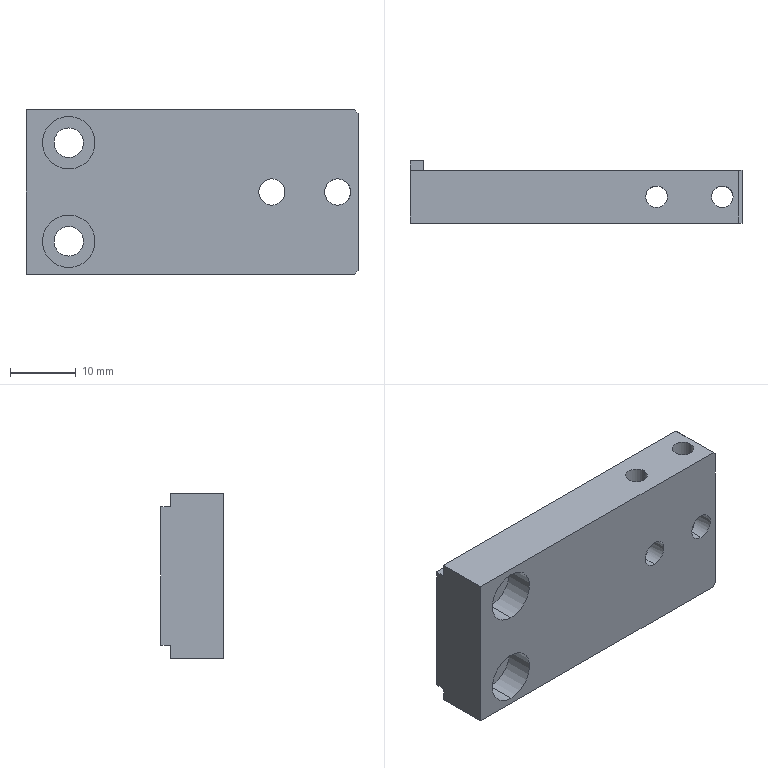Part | STEP file | 11-FG-B07811 | 1 solid | 34 faces | box 50.5 x 9.5 x 25 mm | volume 9037 mm3 | cylinder 20 | plane 14 | commonest cylinder face diameters 3.3 x8 4 x4 4.5 x4 8 x4
STEP:
#1=CARTESIAN_POINT('',(33.85,0.,1.264));
#2=VERTEX_POINT('',#1);
#3=CARTESIAN_POINT('',(35.4,-1.647,2.));
#4=VERTEX_POINT('',#3);
#5=CARTESIAN_POINT('',(33.85,0.,1.264));
#6=CARTESIAN_POINT('',(33.85,-0.2198,1.264));
#7=CARTESIAN_POINT('',(33.895,-0.4332,1.322));
#8=CARTESIAN_POINT('',(34.01,-0.7157,1.439));
#9=CARTESIAN_POINT('',(34.057,-0.8056,1.483));
#10=CARTESIAN_POINT('',(34.163,-0.9726,1.573));
#11=CARTESIAN_POINT('',(34.224,-1.05,1.619));
#12=CARTESIAN_POINT('',(34.358,-1.195,1.709));
#13=CARTESIAN_POINT('',(34.434,-1.263,1.753));
#14=CARTESIAN_POINT('',(34.596,-1.384,1.834));
#15=CARTESIAN_POINT('',(34.684,-1.438,1.87));
#16=CARTESIAN_POINT('',(34.967,-1.575,1.963));
#17=CARTESIAN_POINT('',(35.18,-1.634,2.));
#18=CARTESIAN_POINT('',(35.4,-1.647,2.));
#19=B_SPLINE_CURVE_WITH_KNOTS('',3,(#5,#6,#7,#8,#9,#10,#11,#12,#13,#14,#15,#16,#17,#18),.UNSPECIFIED.,.F.,.F.,(4,2,2,2,2,2,4),(0.008422,0.009072,0.009397,0.009722,0.01005,0.01037,0.01102),.UNSPECIFIED.);
#20=EDGE_CURVE('',#2,#4,#19,.T.);
#21=ORIENTED_EDGE('',*,*,#20,.F.);
#22=CARTESIAN_POINT('',(33.85,0.,12.5));
#23=VERTEX_POINT('',#22);
#24=CARTESIAN_POINT('',(33.85,0.,12.5));
#25=DIRECTION('',(0.,0.,1.));
#26=VECTOR('',#25,1000.);
#27=LINE('',#24,#26);
#28=EDGE_CURVE('',#2,#23,#27,.T.);
#29=ORIENTED_EDGE('',*,*,#28,.T.);
#30=CARTESIAN_POINT('',(37.15,0.,12.5));
#31=VERTEX_POINT('',#30);
#32=CARTESIAN_POINT('',(35.5,0.,12.5));
#33=DIRECTION('',(0.,0.,1.));
#34=DIRECTION('',(1.,0.,0.));
#35=AXIS2_PLACEMENT_3D('',#32,#33,#34);
#36=CIRCLE('',#35,1.65);
#37=EDGE_CURVE('',#23,#31,#36,.T.);
#38=ORIENTED_EDGE('',*,*,#37,.T.);
#39=CARTESIAN_POINT('',(37.15,0.,0.9682));
#40=VERTEX_POINT('',#39);
#41=CARTESIAN_POINT('',(37.15,0.,12.5));
#42=DIRECTION('',(0.,0.,1.));
#43=VECTOR('',#42,1000.);
#44=LINE('',#41,#43);
#45=EDGE_CURVE('',#40,#31,#44,.T.);
#46=ORIENTED_EDGE('',*,*,#45,.F.);
#47=CARTESIAN_POINT('',(35.4,-1.647,2.));
#48=CARTESIAN_POINT('',(35.523,-1.654,2.));
#49=CARTESIAN_POINT('',(35.643,-1.648,1.989));
#50=CARTESIAN_POINT('',(35.88,-1.61,1.945));
#51=CARTESIAN_POINT('',(35.995,-1.578,1.913));
#52=CARTESIAN_POINT('',(36.208,-1.495,1.833));
#53=CARTESIAN_POINT('',(36.309,-1.442,1.784));
#54=CARTESIAN_POINT('',(36.492,-1.323,1.679));
#55=CARTESIAN_POINT('',(36.575,-1.256,1.621));
#56=CARTESIAN_POINT('',(36.726,-1.109,1.5));
#57=CARTESIAN_POINT('',(36.794,-1.029,1.436));
#58=CARTESIAN_POINT('',(36.913,-0.8585,1.311));
#59=CARTESIAN_POINT('',(36.964,-0.7681,1.248));
#60=CARTESIAN_POINT('',(37.051,-0.572,1.131));
#61=CARTESIAN_POINT('',(37.086,-0.4683,1.076));
#62=CARTESIAN_POINT('',(37.136,-0.2428,0.9941));
#63=CARTESIAN_POINT('',(37.15,-0.1222,0.9682));
#64=CARTESIAN_POINT('',(37.15,0.,0.9682));
#65=B_SPLINE_CURVE_WITH_KNOTS('',3,(#47,#48,#49,#50,#51,#52,#53,#54,#55,#56,#57,#58,#59,#60,#61,#62,#63,#64),.UNSPECIFIED.,.F.,.F.,(4,2,2,2,2,2,2,2,4),(0.,0.0003631,0.0007262,0.001089,0.001452,0.001815,0.002179,0.002542,0.002905),.UNSPECIFIED.);
#66=EDGE_CURVE('',#4,#40,#65,.T.);
#67=ORIENTED_EDGE('',*,*,#66,.F.);
#68=EDGE_LOOP('',(#21,#29,#38,#46,#67));
#69=FACE_OUTER_BOUND('',#68,.T.);
#70=CARTESIAN_POINT('',(35.5,0.,12.5));
#71=DIRECTION('',(0.,0.,1.));
#72=DIRECTION('',(1.,0.,0.));
#73=AXIS2_PLACEMENT_3D('',#70,#71,#72);
#74=CYLINDRICAL_SURFACE('',#73,1.65);
#75=ADVANCED_FACE('',(#69),#74,.F.);
#76=CARTESIAN_POINT('',(43.85,0.,1.264));
#77=VERTEX_POINT('',#76);
#78=CARTESIAN_POINT('',(45.4,-1.647,2.));
#79=VERTEX_POINT('',#78);
#80=CARTESIAN_POINT('',(43.85,0.,1.264));
#81=CARTESIAN_POINT('',(43.85,-0.2198,1.264));
#82=CARTESIAN_POINT('',(43.895,-0.4332,1.322));
#83=CARTESIAN_POINT('',(44.01,-0.7157,1.439));
#84=CARTESIAN_POINT('',(44.057,-0.8056,1.483));
#85=CARTESIAN_POINT('',(44.163,-0.9726,1.573));
#86=CARTESIAN_POINT('',(44.224,-1.05,1.619));
#87=CARTESIAN_POINT('',(44.358,-1.195,1.709));
#88=CARTESIAN_POINT('',(44.434,-1.263,1.753));
#89=CARTESIAN_POINT('',(44.596,-1.384,1.834));
#90=CARTESIAN_POINT('',(44.684,-1.438,1.87));
#91=CARTESIAN_POINT('',(44.967,-1.575,1.963));
#92=CARTESIAN_POINT('',(45.18,-1.634,2.));
#93=CARTESIAN_POINT('',(45.4,-1.647,2.));
#94=B_SPLINE_CURVE_WITH_KNOTS('',3,(#80,#81,#82,#83,#84,#85,#86,#87,#88,#89,#90,#91,#92,#93),.UNSPECIFIED.,.F.,.F.,(4,2,2,2,2,2,4),(0.008422,0.009072,0.009397,0.009722,0.01005,0.01037,0.01102),.UNSPECIFIED.);
#95=EDGE_CURVE('',#77,#79,#94,.T.);
#96=ORIENTED_EDGE('',*,*,#95,.F.);
#97=CARTESIAN_POINT('',(43.85,0.,12.5));
#98=VERTEX_POINT('',#97);
#99=CARTESIAN_POINT('',(43.85,0.,12.5));
#100=DIRECTION('',(0.,0.,1.));
#101=VECTOR('',#100,1000.);
#102=LINE('',#99,#101);
#103=EDGE_CURVE('',#77,#98,#102,.T.);
#104=ORIENTED_EDGE('',*,*,#103,.T.);
#105=CARTESIAN_POINT('',(47.15,0.,12.5));
#106=VERTEX_POINT('',#105);
#107=CARTESIAN_POINT('',(45.5,0.,12.5));
#108=DIRECTION('',(0.,0.,1.));
#109=DIRECTION('',(1.,0.,0.));
#110=AXIS2_PLACEMENT_3D('',#107,#108,#109);
#111=CIRCLE('',#110,1.65);
#112=EDGE_CURVE('',#98,#106,#111,.T.);
#113=ORIENTED_EDGE('',*,*,#112,.T.);
#114=CARTESIAN_POINT('',(47.15,0.,0.9682));
#115=VERTEX_POINT('',#114);
#116=CARTESIAN_POINT('',(47.15,0.,12.5));
#117=DIRECTION('',(0.,0.,1.));
#118=VECTOR('',#117,1000.);
#119=LINE('',#116,#118);
#120=EDGE_CURVE('',#115,#106,#119,.T.);
#121=ORIENTED_EDGE('',*,*,#120,.F.);
#122=CARTESIAN_POINT('',(45.4,-1.647,2.));
#123=CARTESIAN_POINT('',(45.523,-1.654,2.));
#124=CARTESIAN_POINT('',(45.643,-1.648,1.989));
#125=CARTESIAN_POINT('',(45.88,-1.61,1.945));
#126=CARTESIAN_POINT('',(45.995,-1.578,1.913));
#127=CARTESIAN_POINT('',(46.208,-1.495,1.833));
#128=CARTESIAN_POINT('',(46.309,-1.442,1.784));
#129=CARTESIAN_POINT('',(46.492,-1.323,1.679));
#130=CARTESIAN_POINT('',(46.575,-1.256,1.621));
#131=CARTESIAN_POINT('',(46.726,-1.109,1.5));
#132=CARTESIAN_POINT('',(46.794,-1.029,1.436));
#133=CARTESIAN_POINT('',(46.913,-0.8585,1.311));
#134=CARTESIAN_POINT('',(46.964,-0.7681,1.248));
#135=CARTESIAN_POINT('',(47.051,-0.572,1.131));
#136=CARTESIAN_POINT('',(47.086,-0.4683,1.076));
#137=CARTESIAN_POINT('',(47.136,-0.2428,0.9941));
#138=CARTESIAN_POINT('',(47.15,-0.1222,0.9682));
#139=CARTESIAN_POINT('',(47.15,0.,0.9682));
#140=B_SPLINE_CURVE_WITH_KNOTS('',3,(#122,#123,#124,#125,#126,#127,#128,#129,#130,#131,#132,#133,#134,#135,#136,#137,#138,#139),.UNSPECIFIED.,.F.,.F.,(4,2,2,2,2,2,2,2,4),(0.,0.0003631,0.0007262,0.001089,0.001452,0.001815,0.002179,0.002542,0.002905),.UNSPECIFIED.);
#141=EDGE_CURVE('',#79,#115,#140,.T.);
#142=ORIENTED_EDGE('',*,*,#141,.F.);
#143=EDGE_LOOP('',(#96,#104,#113,#121,#142));
#144=FACE_OUTER_BOUND('',#143,.T.);
#145=CARTESIAN_POINT('',(45.5,0.,12.5));
#146=DIRECTION('',(0.,0.,1.));
#147=DIRECTION('',(1.,0.,0.));
#148=AXIS2_PLACEMENT_3D('',#145,#146,#147);
#149=CYLINDRICAL_SURFACE('',#148,1.65);
#150=ADVANCED_FACE('',(#144),#149,.F.);
#151=CARTESIAN_POINT('',(37.15,0.,-0.9682));
#152=VERTEX_POINT('',#151);
#153=CARTESIAN_POINT('',(35.4,-1.647,-2.));
#154=VERTEX_POINT('',#153);
#155=CARTESIAN_POINT('',(37.15,0.,-0.9682));
#156=CARTESIAN_POINT('',(37.15,-0.1224,-0.9682));
#157=CARTESIAN_POINT('',(37.136,-0.2437,-0.9944));
#158=CARTESIAN_POINT('',(37.086,-0.4679,-1.076));
#159=CARTESIAN_POINT('',(37.051,-0.5725,-1.131));
#160=CARTESIAN_POINT('',(36.964,-0.7681,-1.248));
#161=CARTESIAN_POINT('',(36.913,-0.8583,-1.311));
#162=CARTESIAN_POINT('',(36.794,-1.029,-1.436));
#163=CARTESIAN_POINT('',(36.726,-1.109,-1.5));
#164=CARTESIAN_POINT('',(36.575,-1.256,-1.621));
#165=CARTESIAN_POINT('',(36.492,-1.323,-1.679));
#166=CARTESIAN_POINT('',(36.31,-1.441,-1.784));
#167=CARTESIAN_POINT('',(36.209,-1.494,-1.832));
#168=CARTESIAN_POINT('',(35.888,-1.62,-1.953));
#169=CARTESIAN_POINT('',(35.643,-1.662,-2.));
#170=CARTESIAN_POINT('',(35.4,-1.647,-2.));
#171=B_SPLINE_CURVE_WITH_KNOTS('',3,(#155,#156,#157,#158,#159,#160,#161,#162,#163,#164,#165,#166,#167,#168,#169,#170),.UNSPECIFIED.,.F.,.F.,(4,2,2,2,2,2,2,4),(0.005499,0.005862,0.006225,0.006589,0.006952,0.007315,0.007678,0.008405),.UNSPECIFIED.);
#172=EDGE_CURVE('',#152,#154,#171,.T.);
#173=ORIENTED_EDGE('',*,*,#172,.F.);
#174=CARTESIAN_POINT('',(37.15,0.,-12.5));
#175=VERTEX_POINT('',#174);
#176=CARTESIAN_POINT('',(37.15,0.,-12.5));
#177=DIRECTION('',(0.,0.,-1.));
#178=VECTOR('',#177,1000.);
#179=LINE('',#176,#178);
#180=EDGE_CURVE('',#152,#175,#179,.T.);
#181=ORIENTED_EDGE('',*,*,#180,.T.);
#182=CARTESIAN_POINT('',(33.85,0.,-12.5));
#183=VERTEX_POINT('',#182);
#184=CARTESIAN_POINT('',(35.5,0.,-12.5));
#185=DIRECTION('',(0.,0.,-1.));
#186=DIRECTION('',(-1.,0.,0.));
#187=AXIS2_PLACEMENT_3D('',#184,#185,#186);
#188=CIRCLE('',#187,1.65);
#189=EDGE_CURVE('',#175,#183,#188,.T.);
#190=ORIENTED_EDGE('',*,*,#189,.T.);
#191=CARTESIAN_POINT('',(33.85,0.,-1.264));
#192=VERTEX_POINT('',#191);
#193=CARTESIAN_POINT('',(33.85,0.,-12.5));
#194=DIRECTION('',(0.,0.,-1.));
#195=VECTOR('',#194,1000.);
#196=LINE('',#193,#195);
#197=EDGE_CURVE('',#192,#183,#196,.T.);
#198=ORIENTED_EDGE('',*,*,#197,.F.);
#199=CARTESIAN_POINT('',(35.4,-1.647,-2.));
#200=CARTESIAN_POINT('',(35.183,-1.634,-2.));
#201=CARTESIAN_POINT('',(34.967,-1.576,-1.963));
#202=CARTESIAN_POINT('',(34.59,-1.392,-1.839));
#203=CARTESIAN_POINT('',(34.426,-1.268,-1.754));
#204=CARTESIAN_POINT('',(34.156,-0.9774,-1.574));
#205=CARTESIAN_POINT('',(34.048,-0.8091,-1.478));
#206=CARTESIAN_POINT('',(33.933,-0.528,-1.361));
#207=CARTESIAN_POINT('',(33.903,-0.4268,-1.326));
#208=CARTESIAN_POINT('',(33.861,-0.2181,-1.278));
#209=CARTESIAN_POINT('',(33.85,-0.1106,-1.264));
#210=CARTESIAN_POINT('',(33.85,0.,-1.264));
#211=B_SPLINE_CURVE_WITH_KNOTS('',3,(#199,#200,#201,#202,#203,#204,#205,#206,#207,#208,#209,#210),.UNSPECIFIED.,.F.,.F.,(4,2,2,2,2,4),(0.008405,0.009054,0.009704,0.01035,0.01068,0.011),.UNSPECIFIED.);
#212=EDGE_CURVE('',#154,#192,#211,.T.);
#213=ORIENTED_EDGE('',*,*,#212,.F.);
#214=EDGE_LOOP('',(#173,#181,#190,#198,#213));
#215=FACE_OUTER_BOUND('',#214,.T.);
#216=CARTESIAN_POINT('',(35.5,0.,-12.5));
#217=DIRECTION('',(0.,0.,-1.));
#218=DIRECTION('',(-1.,0.,0.));
#219=AXIS2_PLACEMENT_3D('',#216,#217,#218);
#220=CYLINDRICAL_SURFACE('',#219,1.65);
#221=ADVANCED_FACE('',(#215),#220,.F.);
#222=CARTESIAN_POINT('',(47.15,0.,-0.9682));
#223=VERTEX_POINT('',#222);
#224=CARTESIAN_POINT('',(45.4,-1.647,-2.));
#225=VERTEX_POINT('',#224);
#226=CARTESIAN_POINT('',(47.15,0.,-0.9682));
#227=CARTESIAN_POINT('',(47.15,-0.1224,-0.9682));
#228=CARTESIAN_POINT('',(47.136,-0.2437,-0.9944));
#229=CARTESIAN_POINT('',(47.086,-0.4679,-1.076));
#230=CARTESIAN_POINT('',(47.051,-0.5725,-1.131));
#231=CARTESIAN_POINT('',(46.964,-0.7681,-1.248));
#232=CARTESIAN_POINT('',(46.913,-0.8583,-1.311));
#233=CARTESIAN_POINT('',(46.794,-1.029,-1.436));
#234=CARTESIAN_POINT('',(46.726,-1.109,-1.5));
#235=CARTESIAN_POINT('',(46.575,-1.256,-1.621));
#236=CARTESIAN_POINT('',(46.492,-1.323,-1.679));
#237=CARTESIAN_POINT('',(46.31,-1.441,-1.784));
#238=CARTESIAN_POINT('',(46.209,-1.494,-1.832));
#239=CARTESIAN_POINT('',(45.888,-1.62,-1.953));
#240=CARTESIAN_POINT('',(45.643,-1.662,-2.));
#241=CARTESIAN_POINT('',(45.4,-1.647,-2.));
#242=B_SPLINE_CURVE_WITH_KNOTS('',3,(#226,#227,#228,#229,#230,#231,#232,#233,#234,#235,#236,#237,#238,#239,#240,#241),.UNSPECIFIED.,.F.,.F.,(4,2,2,2,2,2,2,4),(0.005499,0.005862,0.006225,0.006589,0.006952,0.007315,0.007678,0.008405),.UNSPECIFIED.);
#243=EDGE_CURVE('',#223,#225,#242,.T.);
#244=ORIENTED_EDGE('',*,*,#243,.F.);
#245=CARTESIAN_POINT('',(47.15,0.,-12.5));
#246=VERTEX_POINT('',#245);
#247=CARTESIAN_POINT('',(47.15,0.,-12.5));
#248=DIRECTION('',(0.,0.,-1.));
#249=VECTOR('',#248,1000.);
#250=LINE('',#247,#249);
#251=EDGE_CURVE('',#223,#246,#250,.T.);
#252=ORIENTED_EDGE('',*,*,#251,.T.);
#253=CARTESIAN_POINT('',(43.85,0.,-12.5));
#254=VERTEX_POINT('',#253);
#255=CARTESIAN_POINT('',(45.5,0.,-12.5));
#256=DIRECTION('',(0.,0.,-1.));
#257=DIRECTION('',(-1.,0.,0.));
#258=AXIS2_PLACEMENT_3D('',#255,#256,#257);
#259=CIRCLE('',#258,1.65);
#260=EDGE_CURVE('',#246,#254,#259,.T.);
#261=ORIENTED_EDGE('',*,*,#260,.T.);
#262=CARTESIAN_POINT('',(43.85,0.,-1.264));
#263=VERTEX_POINT('',#262);
#264=CARTESIAN_POINT('',(43.85,0.,-12.5));
#265=DIRECTION('',(0.,0.,-1.));
#266=VECTOR('',#265,1000.);
#267=LINE('',#264,#266);
#268=EDGE_CURVE('',#263,#254,#267,.T.);
#269=ORIENTED_EDGE('',*,*,#268,.F.);
#270=CARTESIAN_POINT('',(45.4,-1.647,-2.));
#271=CARTESIAN_POINT('',(45.183,-1.634,-2.));
#272=CARTESIAN_POINT('',(44.967,-1.576,-1.963));
#273=CARTESIAN_POINT('',(44.59,-1.392,-1.839));
#274=CARTESIAN_POINT('',(44.426,-1.268,-1.754));
#275=CARTESIAN_POINT('',(44.156,-0.9774,-1.574));
#276=CARTESIAN_POINT('',(44.048,-0.8091,-1.478));
#277=CARTESIAN_POINT('',(43.933,-0.528,-1.361));
#278=CARTESIAN_POINT('',(43.903,-0.4268,-1.326));
#279=CARTESIAN_POINT('',(43.861,-0.2181,-1.278));
#280=CARTESIAN_POINT('',(43.85,-0.1106,-1.264));
#281=CARTESIAN_POINT('',(43.85,0.,-1.264));
#282=B_SPLINE_CURVE_WITH_KNOTS('',3,(#270,#271,#272,#273,#274,#275,#276,#277,#278,#279,#280,#281),.UNSPECIFIED.,.F.,.F.,(4,2,2,2,2,4),(0.008405,0.009054,0.009704,0.01035,0.01068,0.011),.UNSPECIFIED.);
#283=EDGE_CURVE('',#225,#263,#282,.T.);
#284=ORIENTED_EDGE('',*,*,#283,.F.);
#285=EDGE_LOOP('',(#244,#252,#261,#269,#284));
#286=FACE_OUTER_BOUND('',#285,.T.);
#287=CARTESIAN_POINT('',(45.5,0.,-12.5));
#288=DIRECTION('',(0.,0.,-1.));
#289=DIRECTION('',(-1.,0.,0.));
#290=AXIS2_PLACEMENT_3D('',#287,#288,#289);
#291=CYLINDRICAL_SURFACE('',#290,1.65);
#292=ADVANCED_FACE('',(#286),#291,.F.);
#293=CARTESIAN_POINT('',(4.5,0.4,11.5));
#294=VERTEX_POINT('',#293);
#295=CARTESIAN_POINT('',(4.5,0.4,3.5));
#296=VERTEX_POINT('',#295);
#297=CARTESIAN_POINT('',(4.5,0.4,7.5));
#298=DIRECTION('',(0.,-1.,0.));
#299=DIRECTION('',(0.,0.,-1.));
#300=AXIS2_PLACEMENT_3D('',#297,#298,#299);
#301=CIRCLE('',#300,4.);
#302=EDGE_CURVE('',#294,#296,#301,.T.);
#303=ORIENTED_EDGE('',*,*,#302,.F.);
#304=CARTESIAN_POINT('',(4.5,-4.,11.5));
#305=VERTEX_POINT('',#304);
#306=CARTESIAN_POINT('',(4.5,-4.,11.5));
#307=DIRECTION('',(0.,-1.,0.));
#308=VECTOR('',#307,1000.);
#309=LINE('',#306,#308);
#310=EDGE_CURVE('',#294,#305,#309,.T.);
#311=ORIENTED_EDGE('',*,*,#310,.T.);
#312=CARTESIAN_POINT('',(4.5,-4.,3.5));
#313=VERTEX_POINT('',#312);
#314=CARTESIAN_POINT('',(4.5,-4.,7.5));
#315=DIRECTION('',(0.,-1.,0.));
#316=DIRECTION('',(0.,0.,-1.));
#317=AXIS2_PLACEMENT_3D('',#314,#315,#316);
#318=CIRCLE('',#317,4.);
#319=EDGE_CURVE('',#305,#313,#318,.T.);
#320=ORIENTED_EDGE('',*,*,#319,.T.);
#321=CARTESIAN_POINT('',(4.5,-4.,3.5));
#322=DIRECTION('',(0.,-1.,0.));
#323=VECTOR('',#322,1000.);
#324=LINE('',#321,#323);
#325=EDGE_CURVE('',#296,#313,#324,.T.);
#326=ORIENTED_EDGE('',*,*,#325,.F.);
#327=EDGE_LOOP('',(#303,#311,#320,#326));
#328=FACE_OUTER_BOUND('',#327,.T.);
#329=CARTESIAN_POINT('',(4.5,-4.,7.5));
#330=DIRECTION('',(0.,-1.,0.));
#331=DIRECTION('',(0.,0.,-1.));
#332=AXIS2_PLACEMENT_3D('',#329,#330,#331);
#333=CYLINDRICAL_SURFACE('',#332,4.);
#334=ADVANCED_FACE('',(#328),#333,.F.);
#335=CARTESIAN_POINT('',(4.5,4.,9.75));
#336=VERTEX_POINT('',#335);
#337=CARTESIAN_POINT('',(4.5,4.,5.25));
#338=VERTEX_POINT('',#337);
#339=CARTESIAN_POINT('',(4.5,4.,7.5));
#340=DIRECTION('',(0.,-1.,0.));
#341=DIRECTION('',(0.,0.,-1.));
#342=AXIS2_PLACEMENT_3D('',#339,#340,#341);
#343=CIRCLE('',#342,2.25);
#344=EDGE_CURVE('',#336,#338,#343,.T.);
#345=ORIENTED_EDGE('',*,*,#344,.F.);
#346=CARTESIAN_POINT('',(4.5,0.4,9.75));
#347=VERTEX_POINT('',#346);
#348=CARTESIAN_POINT('',(4.5,-4.,9.75));
#349=DIRECTION('',(0.,-1.,0.));
#350=VECTOR('',#349,1000.);
#351=LINE('',#348,#350);
#352=EDGE_CURVE('',#336,#347,#351,.T.);
#353=ORIENTED_EDGE('',*,*,#352,.T.);
#354=CARTESIAN_POINT('',(4.5,0.4,5.25));
#355=VERTEX_POINT('',#354);
#356=CARTESIAN_POINT('',(4.5,0.4,7.5));
#357=DIRECTION('',(0.,-1.,0.));
#358=DIRECTION('',(0.,0.,-1.));
#359=AXIS2_PLACEMENT_3D('',#356,#357,#358);
#360=CIRCLE('',#359,2.25);
#361=EDGE_CURVE('',#347,#355,#360,.T.);
#362=ORIENTED_EDGE('',*,*,#361,.T.);
#363=CARTESIAN_POINT('',(4.5,-4.,5.25));
#364=DIRECTION('',(0.,-1.,0.));
#365=VECTOR('',#364,1000.);
#366=LINE('',#363,#365);
#367=EDGE_CURVE('',#338,#355,#366,.T.);
#368=ORIENTED_EDGE('',*,*,#367,.F.);
#369=EDGE_LOOP('',(#345,#353,#362,#368));
#370=FACE_OUTER_BOUND('',#369,.T.);
#371=CARTESIAN_POINT('',(4.5,-4.,7.5));
#372=DIRECTION('',(0.,-1.,0.));
#373=DIRECTION('',(0.,0.,-1.));
#374=AXIS2_PLACEMENT_3D('',#371,#372,#373);
#375=CYLINDRICAL_SURFACE('',#374,2.25);
#376=ADVANCED_FACE('',(#370),#375,.F.);
#377=CARTESIAN_POINT('',(4.5,0.4,-3.5));
#378=VERTEX_POINT('',#377);
#379=CARTESIAN_POINT('',(4.5,0.4,-11.5));
#380=VERTEX_POINT('',#379);
#381=CARTESIAN_POINT('',(4.5,0.4,-7.5));
#382=DIRECTION('',(0.,-1.,0.));
#383=DIRECTION('',(0.,0.,-1.));
#384=AXIS2_PLACEMENT_3D('',#381,#382,#383);
#385=CIRCLE('',#384,4.);
#386=EDGE_CURVE('',#378,#380,#385,.T.);
#387=ORIENTED_EDGE('',*,*,#386,.F.);
#388=CARTESIAN_POINT('',(4.5,-4.,-3.5));
#389=VERTEX_POINT('',#388);
#390=CARTESIAN_POINT('',(4.5,-4.,-3.5));
#391=DIRECTION('',(0.,-1.,0.));
#392=VECTOR('',#391,1000.);
#393=LINE('',#390,#392);
#394=EDGE_CURVE('',#378,#389,#393,.T.);
#395=ORIENTED_EDGE('',*,*,#394,.T.);
#396=CARTESIAN_POINT('',(4.5,-4.,-11.5));
#397=VERTEX_POINT('',#396);
#398=CARTESIAN_POINT('',(4.5,-4.,-7.5));
#399=DIRECTION('',(0.,-1.,0.));
#400=DIRECTION('',(0.,0.,-1.));
#401=AXIS2_PLACEMENT_3D('',#398,#399,#400);
#402=CIRCLE('',#401,4.);
#403=EDGE_CURVE('',#389,#397,#402,.T.);
#404=ORIENTED_EDGE('',*,*,#403,.T.);
#405=CARTESIAN_POINT('',(4.5,-4.,-11.5));
#406=DIRECTION('',(0.,-1.,0.));
#407=VECTOR('',#406,1000.);
#408=LINE('',#405,#407);
#409=EDGE_CURVE('',#380,#397,#408,.T.);
#410=ORIENTED_EDGE('',*,*,#409,.F.);
#411=EDGE_LOOP('',(#387,#395,#404,#410));
#412=FACE_OUTER_BOUND('',#411,.T.);
#413=CARTESIAN_POINT('',(4.5,-4.,-7.5));
#414=DIRECTION('',(0.,-1.,0.));
#415=DIRECTION('',(0.,0.,-1.));
#416=AXIS2_PLACEMENT_3D('',#413,#414,#415);
#417=CYLINDRICAL_SURFACE('',#416,4.);
#418=ADVANCED_FACE('',(#412),#417,.F.);
#419=CARTESIAN_POINT('',(4.5,4.,-5.25));
#420=VERTEX_POINT('',#419);
#421=CARTESIAN_POINT('',(4.5,4.,-9.75));
#422=VERTEX_POINT('',#421);
#423=CARTESIAN_POINT('',(4.5,4.,-7.5));
#424=DIRECTION('',(0.,-1.,0.));
#425=DIRECTION('',(0.,0.,-1.));
#426=AXIS2_PLACEMENT_3D('',#423,#424,#425);
#427=CIRCLE('',#426,2.25);
#428=EDGE_CURVE('',#420,#422,#427,.T.);
#429=ORIENTED_EDGE('',*,*,#428,.F.);
#430=CARTESIAN_POINT('',(4.5,0.4,-5.25));
#431=VERTEX_POINT('',#430);
#432=CARTESIAN_POINT('',(4.5,-4.,-5.25));
#433=DIRECTION('',(0.,-1.,0.));
#434=VECTOR('',#433,1000.);
#435=LINE('',#432,#434);
#436=EDGE_CURVE('',#420,#431,#435,.T.);
#437=ORIENTED_EDGE('',*,*,#436,.T.);
#438=CARTESIAN_POINT('',(4.5,0.4,-9.75));
#439=VERTEX_POINT('',#438);
#440=CARTESIAN_POINT('',(4.5,0.4,-7.5));
#441=DIRECTION('',(0.,-1.,0.));
#442=DIRECTION('',(0.,0.,-1.));
#443=AXIS2_PLACEMENT_3D('',#440,#441,#442);
#444=CIRCLE('',#443,2.25);
#445=EDGE_CURVE('',#431,#439,#444,.T.);
#446=ORIENTED_EDGE('',*,*,#445,.T.);
#447=CARTESIAN_POINT('',(4.5,-4.,-9.75));
#448=DIRECTION('',(0.,-1.,0.));
#449=VECTOR('',#448,1000.);
#450=LINE('',#447,#449);
#451=EDGE_CURVE('',#422,#439,#450,.T.);
#452=ORIENTED_EDGE('',*,*,#451,.F.);
#453=EDGE_LOOP('',(#429,#437,#446,#452));
#454=FACE_OUTER_BOUND('',#453,.T.);
#455=CARTESIAN_POINT('',(4.5,-4.,-7.5));
#456=DIRECTION('',(0.,-1.,0.));
#457=DIRECTION('',(0.,0.,-1.));
#458=AXIS2_PLACEMENT_3D('',#455,#456,#457);
#459=CYLINDRICAL_SURFACE('',#458,2.25);
#460=ADVANCED_FACE('',(#454),#459,.F.);
#461=CARTESIAN_POINT('',(35.4,-4.,-2.));
#462=VERTEX_POINT('',#461);
#463=CARTESIAN_POINT('',(35.4,-4.,2.));
#464=VERTEX_POINT('',#463);
#465=CARTESIAN_POINT('',(35.4,-4.,0.));
#466=DIRECTION('',(0.,1.,0.));
#467=DIRECTION('',(0.,0.,1.));
#468=AXIS2_PLACEMENT_3D('',#465,#466,#467);
#469=CIRCLE('',#468,2.);
#470=EDGE_CURVE('',#462,#464,#469,.T.);
#471=ORIENTED_EDGE('',*,*,#470,.F.);
#472=CARTESIAN_POINT('',(35.4,-11.,-2.));
#473=DIRECTION('',(0.,1.,0.));
#474=VECTOR('',#473,1000.);
#475=LINE('',#472,#474);
#476=EDGE_CURVE('',#462,#154,#475,.T.);
#477=ORIENTED_EDGE('',*,*,#476,.T.);
#478=ORIENTED_EDGE('',*,*,#212,.T.);
#479=CARTESIAN_POINT('',(35.4,1.647,-2.));
#480=VERTEX_POINT('',#479);
#481=CARTESIAN_POINT('',(33.85,0.,-1.264));
#482=CARTESIAN_POINT('',(33.85,0.1109,-1.264));
#483=CARTESIAN_POINT('',(33.861,0.218,-1.278));
#484=CARTESIAN_POINT('',(33.902,0.4262,-1.326));
#485=CARTESIAN_POINT('',(33.933,0.5276,-1.361));
#486=CARTESIAN_POINT('',(34.048,0.81,-1.478));
#487=CARTESIAN_POINT('',(34.157,0.9788,-1.575));
#488=CARTESIAN_POINT('',(34.427,1.269,-1.755));
#489=CARTESIAN_POINT('',(34.592,1.393,-1.84));
#490=CARTESIAN_POINT('',(34.874,1.53,-1.932));
#491=CARTESIAN_POINT('',(34.976,1.568,-1.957));
#492=CARTESIAN_POINT('',(35.184,1.623,-1.991));
#493=CARTESIAN_POINT('',(35.29,1.64,-2.));
#494=CARTESIAN_POINT('',(35.4,1.647,-2.));
#495=B_SPLINE_CURVE_WITH_KNOTS('',3,(#481,#482,#483,#484,#485,#486,#487,#488,#489,#490,#491,#492,#493,#494),.UNSPECIFIED.,.F.,.F.,(4,2,2,2,2,2,4),(0.,0.0003254,0.0006508,0.001302,0.001952,0.002278,0.002603),.UNSPECIFIED.);
#496=EDGE_CURVE('',#192,#480,#495,.T.);
#497=ORIENTED_EDGE('',*,*,#496,.T.);
#498=CARTESIAN_POINT('',(35.4,4.,-2.));
#499=VERTEX_POINT('',#498);
#500=CARTESIAN_POINT('',(35.4,-11.,-2.));
#501=DIRECTION('',(0.,1.,0.));
#502=VECTOR('',#501,1000.);
#503=LINE('',#500,#502);
#504=EDGE_CURVE('',#480,#499,#503,.T.);
#505=ORIENTED_EDGE('',*,*,#504,.T.);
#506=CARTESIAN_POINT('',(35.4,4.,2.));
#507=VERTEX_POINT('',#506);
#508=CARTESIAN_POINT('',(35.4,4.,0.));
#509=DIRECTION('',(0.,1.,0.));
#510=DIRECTION('',(0.,0.,1.));
#511=AXIS2_PLACEMENT_3D('',#508,#509,#510);
#512=CIRCLE('',#511,2.);
#513=EDGE_CURVE('',#499,#507,#512,.T.);
#514=ORIENTED_EDGE('',*,*,#513,.T.);
#515=CARTESIAN_POINT('',(35.4,1.647,2.));
#516=VERTEX_POINT('',#515);
#517=CARTESIAN_POINT('',(35.4,-11.,2.));
#518=DIRECTION('',(0.,1.,0.));
#519=VECTOR('',#518,1000.);
#520=LINE('',#517,#519);
#521=EDGE_CURVE('',#516,#507,#520,.T.);
#522=ORIENTED_EDGE('',*,*,#521,.F.);
#523=CARTESIAN_POINT('',(35.4,1.647,2.));
#524=CARTESIAN_POINT('',(35.291,1.64,2.));
#525=CARTESIAN_POINT('',(35.182,1.623,1.991));
#526=CARTESIAN_POINT('',(34.974,1.568,1.957));
#527=CARTESIAN_POINT('',(34.873,1.53,1.932));
#528=CARTESIAN_POINT('',(34.59,1.393,1.84));
#529=CARTESIAN_POINT('',(34.426,1.268,1.754));
#530=CARTESIAN_POINT('',(34.156,0.978,1.575));
#531=CARTESIAN_POINT('',(34.048,0.8097,1.478));
#532=CARTESIAN_POINT('',(33.896,0.4355,1.323));
#533=CARTESIAN_POINT('',(33.85,0.2201,1.264));
#534=CARTESIAN_POINT('',(33.85,0.,1.264));
#535=B_SPLINE_CURVE_WITH_KNOTS('',3,(#523,#524,#525,#526,#527,#528,#529,#530,#531,#532,#533,#534),.UNSPECIFIED.,.F.,.F.,(4,2,2,2,2,4),(0.005819,0.006144,0.00647,0.007121,0.007771,0.008422),.UNSPECIFIED.);
#536=EDGE_CURVE('',#516,#2,#535,.T.);
#537=ORIENTED_EDGE('',*,*,#536,.T.);
#538=ORIENTED_EDGE('',*,*,#20,.T.);
#539=CARTESIAN_POINT('',(35.4,-11.,2.));
#540=DIRECTION('',(0.,1.,0.));
#541=VECTOR('',#540,1000.);
#542=LINE('',#539,#541);
#543=EDGE_CURVE('',#464,#4,#542,.T.);
#544=ORIENTED_EDGE('',*,*,#543,.F.);
#545=EDGE_LOOP('',(#471,#477,#478,#497,#505,#514,#522,#537,#538,#544));
#546=FACE_OUTER_BOUND('',#545,.T.);
#547=CARTESIAN_POINT('',(35.4,-11.,0.));
#548=DIRECTION('',(0.,1.,0.));
#549=DIRECTION('',(0.,0.,1.));
#550=AXIS2_PLACEMENT_3D('',#547,#548,#549);
#551=CYLINDRICAL_SURFACE('',#550,2.);
#552=ADVANCED_FACE('',(#546),#551,.F.);
#553=CARTESIAN_POINT('',(45.4,-4.,-2.));
#554=VERTEX_POINT('',#553);
#555=CARTESIAN_POINT('',(45.4,-4.,2.));
#556=VERTEX_POINT('',#555);
#557=CARTESIAN_POINT('',(45.4,-4.,0.));
#558=DIRECTION('',(0.,1.,0.));
#559=DIRECTION('',(0.,0.,1.));
#560=AXIS2_PLACEMENT_3D('',#557,#558,#559);
#561=CIRCLE('',#560,2.);
#562=EDGE_CURVE('',#554,#556,#561,.T.);
#563=ORIENTED_EDGE('',*,*,#562,.F.);
#564=CARTESIAN_POINT('',(45.4,-11.,-2.));
#565=DIRECTION('',(0.,1.,0.));
#566=VECTOR('',#565,1000.);
#567=LINE('',#564,#566);
#568=EDGE_CURVE('',#554,#225,#567,.T.);
#569=ORIENTED_EDGE('',*,*,#568,.T.);
#570=ORIENTED_EDGE('',*,*,#283,.T.);
#571=CARTESIAN_POINT('',(45.4,1.647,-2.));
#572=VERTEX_POINT('',#571);
#573=CARTESIAN_POINT('',(43.85,0.,-1.264));
#574=CARTESIAN_POINT('',(43.85,0.1109,-1.264));
#575=CARTESIAN_POINT('',(43.861,0.218,-1.278));
#576=CARTESIAN_POINT('',(43.902,0.4262,-1.326));
#577=CARTESIAN_POINT('',(43.933,0.5276,-1.361));
#578=CARTESIAN_POINT('',(44.048,0.81,-1.478));
#579=CARTESIAN_POINT('',(44.157,0.9788,-1.575));
#580=CARTESIAN_POINT('',(44.427,1.269,-1.755));
#581=CARTESIAN_POINT('',(44.592,1.393,-1.84));
#582=CARTESIAN_POINT('',(44.874,1.53,-1.932));
#583=CARTESIAN_POINT('',(44.976,1.568,-1.957));
#584=CARTESIAN_POINT('',(45.184,1.623,-1.991));
#585=CARTESIAN_POINT('',(45.29,1.64,-2.));
#586=CARTESIAN_POINT('',(45.4,1.647,-2.));
#587=B_SPLINE_CURVE_WITH_KNOTS('',3,(#573,#574,#575,#576,#577,#578,#579,#580,#581,#582,#583,#584,#585,#586),.UNSPECIFIED.,.F.,.F.,(4,2,2,2,2,2,4),(0.,0.0003254,0.0006508,0.001302,0.001952,0.002278,0.002603),.UNSPECIFIED.);
#588=EDGE_CURVE('',#263,#572,#587,.T.);
#589=ORIENTED_EDGE('',*,*,#588,.T.);
#590=CARTESIAN_POINT('',(45.4,4.,-2.));
#591=VERTEX_POINT('',#590);
#592=CARTESIAN_POINT('',(45.4,-11.,-2.));
#593=DIRECTION('',(0.,1.,0.));
#594=VECTOR('',#593,1000.);
#595=LINE('',#592,#594);
#596=EDGE_CURVE('',#572,#591,#595,.T.);
#597=ORIENTED_EDGE('',*,*,#596,.T.);
#598=CARTESIAN_POINT('',(45.4,4.,2.));
#599=VERTEX_POINT('',#598);
#600=CARTESIAN_POINT('',(45.4,4.,0.));
#601=DIRECTION('',(0.,1.,0.));
#602=DIRECTION('',(0.,0.,1.));
#603=AXIS2_PLACEMENT_3D('',#600,#601,#602);
#604=CIRCLE('',#603,2.);
#605=EDGE_CURVE('',#591,#599,#604,.T.);
#606=ORIENTED_EDGE('',*,*,#605,.T.);
#607=CARTESIAN_POINT('',(45.4,1.647,2.));
#608=VERTEX_POINT('',#607);
#609=CARTESIAN_POINT('',(45.4,-11.,2.));
#610=DIRECTION('',(0.,1.,0.));
#611=VECTOR('',#610,1000.);
#612=LINE('',#609,#611);
#613=EDGE_CURVE('',#608,#599,#612,.T.);
#614=ORIENTED_EDGE('',*,*,#613,.F.);
#615=CARTESIAN_POINT('',(45.4,1.647,2.));
#616=CARTESIAN_POINT('',(45.291,1.64,2.));
#617=CARTESIAN_POINT('',(45.182,1.623,1.991));
#618=CARTESIAN_POINT('',(44.974,1.568,1.957));
#619=CARTESIAN_POINT('',(44.873,1.53,1.932));
#620=CARTESIAN_POINT('',(44.59,1.393,1.84));
#621=CARTESIAN_POINT('',(44.426,1.268,1.754));
#622=CARTESIAN_POINT('',(44.156,0.978,1.575));
#623=CARTESIAN_POINT('',(44.048,0.8097,1.478));
#624=CARTESIAN_POINT('',(43.896,0.4355,1.323));
#625=CARTESIAN_POINT('',(43.85,0.2201,1.264));
#626=CARTESIAN_POINT('',(43.85,0.,1.264));
#627=B_SPLINE_CURVE_WITH_KNOTS('',3,(#615,#616,#617,#618,#619,#620,#621,#622,#623,#624,#625,#626),.UNSPECIFIED.,.F.,.F.,(4,2,2,2,2,4),(0.005819,0.006144,0.00647,0.007121,0.007771,0.008422),.UNSPECIFIED.);
#628=EDGE_CURVE('',#608,#77,#627,.T.);
#629=ORIENTED_EDGE('',*,*,#628,.T.);
#630=ORIENTED_EDGE('',*,*,#95,.T.);
#631=CARTESIAN_POINT('',(45.4,-11.,2.));
#632=DIRECTION('',(0.,1.,0.));
#633=VECTOR('',#632,1000.);
#634=LINE('',#631,#633);
#635=EDGE_CURVE('',#556,#79,#634,.T.);
#636=ORIENTED_EDGE('',*,*,#635,.F.);
#637=EDGE_LOOP('',(#563,#569,#570,#589,#597,#606,#614,#629,#630,#636));
#638=FACE_OUTER_BOUND('',#637,.T.);
#639=CARTESIAN_POINT('',(45.4,-11.,0.));
#640=DIRECTION('',(0.,1.,0.));
#641=DIRECTION('',(0.,0.,1.));
#642=AXIS2_PLACEMENT_3D('',#639,#640,#641);
#643=CYLINDRICAL_SURFACE('',#642,2.);
#644=ADVANCED_FACE('',(#638),#643,.F.);
#645=CARTESIAN_POINT('',(35.5,0.,12.5));
#646=DIRECTION('',(0.,0.,1.));
#647=DIRECTION('',(1.,0.,0.));
#648=AXIS2_PLACEMENT_3D('',#645,#646,#647);
#649=CIRCLE('',#648,1.65);
#650=EDGE_CURVE('',#31,#23,#649,.T.);
#651=ORIENTED_EDGE('',*,*,#650,.F.);
#652=ORIENTED_EDGE('',*,*,#37,.F.);
#653=EDGE_LOOP('',(#651,#652));
#654=FACE_BOUND('',#653,.T.);
#655=CARTESIAN_POINT('',(45.5,0.,12.5));
#656=DIRECTION('',(0.,0.,1.));
#657=DIRECTION('',(1.,0.,0.));
#658=AXIS2_PLACEMENT_3D('',#655,#656,#657);
#659=CIRCLE('',#658,1.65);
#660=EDGE_CURVE('',#106,#98,#659,.T.);
#661=ORIENTED_EDGE('',*,*,#660,.F.);
#662=ORIENTED_EDGE('',*,*,#112,.F.);
#663=EDGE_LOOP('',(#661,#662));
#664=FACE_BOUND('',#663,.T.);
#665=CARTESIAN_POINT('',(48.,4.,12.5));
#666=VERTEX_POINT('',#665);
#667=CARTESIAN_POINT('',(-2.,4.,12.5));
#668=VERTEX_POINT('',#667);
#669=CARTESIAN_POINT('',(48.5,4.,12.5));
#670=DIRECTION('',(-1.,0.,0.));
#671=VECTOR('',#670,1000.);
#672=LINE('',#669,#671);
#673=EDGE_CURVE('',#666,#668,#672,.T.);
#674=ORIENTED_EDGE('',*,*,#673,.T.);
#675=CARTESIAN_POINT('',(-2.,-4.,12.5));
#676=VERTEX_POINT('',#675);
#677=CARTESIAN_POINT('',(-2.,-4.,12.5));
#678=DIRECTION('',(0.,-1.,0.));
#679=VECTOR('',#678,1000.);
#680=LINE('',#677,#679);
#681=EDGE_CURVE('',#668,#676,#680,.T.);
#682=ORIENTED_EDGE('',*,*,#681,.T.);
#683=CARTESIAN_POINT('',(48.,-4.,12.5));
#684=VERTEX_POINT('',#683);
#685=CARTESIAN_POINT('',(48.5,-4.,12.5));
#686=DIRECTION('',(-1.,0.,0.));
#687=VECTOR('',#686,1000.);
#688=LINE('',#685,#687);
#689=EDGE_CURVE('',#684,#676,#688,.T.);
#690=ORIENTED_EDGE('',*,*,#689,.F.);
#691=CARTESIAN_POINT('',(48.,4.,12.5));
#692=DIRECTION('',(0.,1.,0.));
#693=VECTOR('',#692,1000.);
#694=LINE('',#691,#693);
#695=EDGE_CURVE('',#684,#666,#694,.T.);
#696=ORIENTED_EDGE('',*,*,#695,.T.);
#697=EDGE_LOOP('',(#674,#682,#690,#696));
#698=FACE_OUTER_BOUND('',#697,.T.);
#699=CARTESIAN_POINT('',(48.5,-4.,12.5));
#700=DIRECTION('',(0.,0.,-1.));
#701=DIRECTION('',(-1.,0.,0.));
#702=AXIS2_PLACEMENT_3D('',#699,#700,#701);
#703=PLANE('',#702);
#704=ADVANCED_FACE('',(#654,#664,#698),#703,.F.);
#705=CARTESIAN_POINT('',(4.5,-4.,7.5));
#706=DIRECTION('',(0.,-1.,0.));
#707=DIRECTION('',(0.,0.,-1.));
#708=AXIS2_PLACEMENT_3D('',#705,#706,#707);
#709=CIRCLE('',#708,4.);
#710=EDGE_CURVE('',#313,#305,#709,.T.);
#711=ORIENTED_EDGE('',*,*,#710,.F.);
#712=ORIENTED_EDGE('',*,*,#319,.F.);
#713=EDGE_LOOP('',(#711,#712));
#714=FACE_BOUND('',#713,.T.);
#715=CARTESIAN_POINT('',(4.5,-4.,-7.5));
#716=DIRECTION('',(0.,-1.,0.));
#717=DIRECTION('',(0.,0.,-1.));
#718=AXIS2_PLACEMENT_3D('',#715,#716,#717);
#719=CIRCLE('',#718,4.);
#720=EDGE_CURVE('',#397,#389,#719,.T.);
#721=ORIENTED_EDGE('',*,*,#720,.F.);
#722=ORIENTED_EDGE('',*,*,#403,.F.);
#723=EDGE_LOOP('',(#721,#722));
#724=FACE_BOUND('',#723,.T.);
#725=CARTESIAN_POINT('',(35.4,-4.,0.));
#726=DIRECTION('',(0.,1.,0.));
#727=DIRECTION('',(0.,0.,1.));
#728=AXIS2_PLACEMENT_3D('',#725,#726,#727);
#729=CIRCLE('',#728,2.);
#730=EDGE_CURVE('',#464,#462,#729,.T.);
#731=ORIENTED_EDGE('',*,*,#730,.T.);
#732=ORIENTED_EDGE('',*,*,#470,.T.);
#733=EDGE_LOOP('',(#731,#732));
#734=FACE_BOUND('',#733,.T.);
#735=CARTESIAN_POINT('',(45.4,-4.,0.));
#736=DIRECTION('',(0.,1.,0.));
#737=DIRECTION('',(0.,0.,1.));
#738=AXIS2_PLACEMENT_3D('',#735,#736,#737);
#739=CIRCLE('',#738,2.);
#740=EDGE_CURVE('',#556,#554,#739,.T.);
#741=ORIENTED_EDGE('',*,*,#740,.T.);
#742=ORIENTED_EDGE('',*,*,#562,.T.);
#743=EDGE_LOOP('',(#741,#742));
#744=FACE_BOUND('',#743,.T.);
#745=CARTESIAN_POINT('',(48.,-4.,-12.5));
#746=VERTEX_POINT('',#745);
#747=CARTESIAN_POINT('',(-2.,-4.,-12.5));
#748=VERTEX_POINT('',#747);
#749=CARTESIAN_POINT('',(48.5,-4.,-12.5));
#750=DIRECTION('',(-1.,0.,0.));
#751=VECTOR('',#750,1000.);
#752=LINE('',#749,#751);
#753=EDGE_CURVE('',#746,#748,#752,.T.);
#754=ORIENTED_EDGE('',*,*,#753,.F.);
#755=CARTESIAN_POINT('',(48.5,-4.,-12.));
#756=VERTEX_POINT('',#755);
#757=CARTESIAN_POINT('',(48.5,-4.,-12.));
#758=DIRECTION('',(0.7071,0.,0.7071));
#759=VECTOR('',#758,1000.);
#760=LINE('',#757,#759);
#761=EDGE_CURVE('',#746,#756,#760,.T.);
#762=ORIENTED_EDGE('',*,*,#761,.T.);
#763=CARTESIAN_POINT('',(48.5,-4.,12.));
#764=VERTEX_POINT('',#763);
#765=CARTESIAN_POINT('',(48.5,-4.,-12.5));
#766=DIRECTION('',(0.,0.,-1.));
#767=VECTOR('',#766,1000.);
#768=LINE('',#765,#767);
#769=EDGE_CURVE('',#764,#756,#768,.T.);
#770=ORIENTED_EDGE('',*,*,#769,.F.);
#771=CARTESIAN_POINT('',(48.5,-4.,12.));
#772=DIRECTION('',(-0.7071,0.,0.7071));
#773=VECTOR('',#772,1000.);
#774=LINE('',#771,#773);
#775=EDGE_CURVE('',#764,#684,#774,.T.);
#776=ORIENTED_EDGE('',*,*,#775,.T.);
#777=ORIENTED_EDGE('',*,*,#689,.T.);
#778=CARTESIAN_POINT('',(-2.,-4.,-22.208));
#779=DIRECTION('',(0.,0.,1.));
#780=VECTOR('',#779,1000.);
#781=LINE('',#778,#780);
#782=EDGE_CURVE('',#748,#676,#781,.T.);
#783=ORIENTED_EDGE('',*,*,#782,.F.);
#784=EDGE_LOOP('',(#754,#762,#770,#776,#777,#783));
#785=FACE_OUTER_BOUND('',#784,.T.);
#786=CARTESIAN_POINT('',(48.5,-4.,-12.5));
#787=DIRECTION('',(0.,1.,0.));
#788=DIRECTION('',(0.,0.,1.));
#789=AXIS2_PLACEMENT_3D('',#786,#787,#788);
#790=PLANE('',#789);
#791=ADVANCED_FACE('',(#714,#724,#734,#744,#785),#790,.F.);
#792=CARTESIAN_POINT('',(35.5,0.,-12.5));
#793=DIRECTION('',(0.,0.,-1.));
#794=DIRECTION('',(-1.,0.,0.));
#795=AXIS2_PLACEMENT_3D('',#792,#793,#794);
#796=CIRCLE('',#795,1.65);
#797=EDGE_CURVE('',#183,#175,#796,.T.);
#798=ORIENTED_EDGE('',*,*,#797,.F.);
#799=ORIENTED_EDGE('',*,*,#189,.F.);
#800=EDGE_LOOP('',(#798,#799));
#801=FACE_BOUND('',#800,.T.);
#802=CARTESIAN_POINT('',(45.5,0.,-12.5));
#803=DIRECTION('',(0.,0.,-1.));
#804=DIRECTION('',(-1.,0.,0.));
#805=AXIS2_PLACEMENT_3D('',#802,#803,#804);
#806=CIRCLE('',#805,1.65);
#807=EDGE_CURVE('',#254,#246,#806,.T.);
#808=ORIENTED_EDGE('',*,*,#807,.F.);
#809=ORIENTED_EDGE('',*,*,#260,.F.);
#810=EDGE_LOOP('',(#808,#809));
#811=FACE_BOUND('',#810,.T.);
#812=CARTESIAN_POINT('',(-2.,4.,-12.5));
#813=VERTEX_POINT('',#812);
#814=CARTESIAN_POINT('',(-2.,-4.,-12.5));
#815=DIRECTION('',(0.,1.,0.));
#816=VECTOR('',#815,1000.);
#817=LINE('',#814,#816);
#818=EDGE_CURVE('',#748,#813,#817,.T.);
#819=ORIENTED_EDGE('',*,*,#818,.T.);
#820=CARTESIAN_POINT('',(48.,4.,-12.5));
#821=VERTEX_POINT('',#820);
#822=CARTESIAN_POINT('',(48.5,4.,-12.5));
#823=DIRECTION('',(-1.,0.,0.));
#824=VECTOR('',#823,1000.);
#825=LINE('',#822,#824);
#826=EDGE_CURVE('',#821,#813,#825,.T.);
#827=ORIENTED_EDGE('',*,*,#826,.F.);
#828=CARTESIAN_POINT('',(48.,-4.,-12.5));
#829=DIRECTION('',(0.,-1.,0.));
#830=VECTOR('',#829,1000.);
#831=LINE('',#828,#830);
#832=EDGE_CURVE('',#821,#746,#831,.T.);
#833=ORIENTED_EDGE('',*,*,#832,.T.);
#834=ORIENTED_EDGE('',*,*,#753,.T.);
#835=EDGE_LOOP('',(#819,#827,#833,#834));
#836=FACE_OUTER_BOUND('',#835,.T.);
#837=CARTESIAN_POINT('',(48.5,-4.,-12.5));
#838=DIRECTION('',(0.,0.,1.));
#839=DIRECTION('',(1.,0.,0.));
#840=AXIS2_PLACEMENT_3D('',#837,#838,#839);
#841=PLANE('',#840);
#842=ADVANCED_FACE('',(#801,#811,#836),#841,.F.);
#843=CARTESIAN_POINT('',(4.5,4.,7.5));
#844=DIRECTION('',(0.,-1.,0.));
#845=DIRECTION('',(0.,0.,-1.));
#846=AXIS2_PLACEMENT_3D('',#843,#844,#845);
#847=CIRCLE('',#846,2.25);
#848=EDGE_CURVE('',#338,#336,#847,.T.);
#849=ORIENTED_EDGE('',*,*,#848,.T.);
#850=ORIENTED_EDGE('',*,*,#344,.T.);
#851=EDGE_LOOP('',(#849,#850));
#852=FACE_BOUND('',#851,.T.);
#853=CARTESIAN_POINT('',(4.5,4.,-7.5));
#854=DIRECTION('',(0.,-1.,0.));
#855=DIRECTION('',(0.,0.,-1.));
#856=AXIS2_PLACEMENT_3D('',#853,#854,#855);
#857=CIRCLE('',#856,2.25);
#858=EDGE_CURVE('',#422,#420,#857,.T.);
#859=ORIENTED_EDGE('',*,*,#858,.T.);
#860=ORIENTED_EDGE('',*,*,#428,.T.);
#861=EDGE_LOOP('',(#859,#860));
#862=FACE_BOUND('',#861,.T.);
#863=CARTESIAN_POINT('',(35.4,4.,0.));
#864=DIRECTION('',(0.,1.,0.));
#865=DIRECTION('',(0.,0.,1.));
#866=AXIS2_PLACEMENT_3D('',#863,#864,#865);
#867=CIRCLE('',#866,2.);
#868=EDGE_CURVE('',#507,#499,#867,.T.);
#869=ORIENTED_EDGE('',*,*,#868,.F.);
#870=ORIENTED_EDGE('',*,*,#513,.F.);
#871=EDGE_LOOP('',(#869,#870));
#872=FACE_BOUND('',#871,.T.);
#873=CARTESIAN_POINT('',(45.4,4.,0.));
#874=DIRECTION('',(0.,1.,0.));
#875=DIRECTION('',(0.,0.,1.));
#876=AXIS2_PLACEMENT_3D('',#873,#874,#875);
#877=CIRCLE('',#876,2.);
#878=EDGE_CURVE('',#599,#591,#877,.T.);
#879=ORIENTED_EDGE('',*,*,#878,.F.);
#880=ORIENTED_EDGE('',*,*,#605,.F.);
#881=EDGE_LOOP('',(#879,#880));
#882=FACE_BOUND('',#881,.T.);
#883=CARTESIAN_POINT('',(48.5,4.,-12.));
#884=VERTEX_POINT('',#883);
#885=CARTESIAN_POINT('',(48.5,4.,12.));
#886=VERTEX_POINT('',#885);
#887=CARTESIAN_POINT('',(48.5,4.,-12.5));
#888=DIRECTION('',(0.,0.,1.));
#889=VECTOR('',#888,1000.);
#890=LINE('',#887,#889);
#891=EDGE_CURVE('',#884,#886,#890,.T.);
#892=ORIENTED_EDGE('',*,*,#891,.F.);
#893=CARTESIAN_POINT('',(48.5,4.,-12.));
#894=DIRECTION('',(-0.7071,0.,-0.7071));
#895=VECTOR('',#894,1000.);
#896=LINE('',#893,#895);
#897=EDGE_CURVE('',#884,#821,#896,.T.);
#898=ORIENTED_EDGE('',*,*,#897,.T.);
#899=ORIENTED_EDGE('',*,*,#826,.T.);
#900=CARTESIAN_POINT('',(-2.,4.,-10.5));
#901=VERTEX_POINT('',#900);
#902=CARTESIAN_POINT('',(-2.,4.,-22.208));
#903=DIRECTION('',(0.,0.,1.));
#904=VECTOR('',#903,1000.);
#905=LINE('',#902,#904);
#906=EDGE_CURVE('',#813,#901,#905,.T.);
#907=ORIENTED_EDGE('',*,*,#906,.T.);
#908=CARTESIAN_POINT('',(0.,4.,-10.5));
#909=VERTEX_POINT('',#908);
#910=CARTESIAN_POINT('',(-10.,4.,-10.5));
#911=DIRECTION('',(1.,0.,0.));
#912=VECTOR('',#911,1000.);
#913=LINE('',#910,#912);
#914=EDGE_CURVE('',#901,#909,#913,.T.);
#915=ORIENTED_EDGE('',*,*,#914,.T.);
#916=CARTESIAN_POINT('',(0.,4.,10.5));
#917=VERTEX_POINT('',#916);
#918=CARTESIAN_POINT('',(0.,4.,-12.5));
#919=DIRECTION('',(0.,0.,1.));
#920=VECTOR('',#919,1000.);
#921=LINE('',#918,#920);
#922=EDGE_CURVE('',#909,#917,#921,.T.);
#923=ORIENTED_EDGE('',*,*,#922,.T.);
#924=CARTESIAN_POINT('',(-2.,4.,10.5));
#925=VERTEX_POINT('',#924);
#926=CARTESIAN_POINT('',(-10.,4.,10.5));
#927=DIRECTION('',(1.,0.,0.));
#928=VECTOR('',#927,1000.);
#929=LINE('',#926,#928);
#930=EDGE_CURVE('',#925,#917,#929,.T.);
#931=ORIENTED_EDGE('',*,*,#930,.F.);
#932=CARTESIAN_POINT('',(-2.,4.,-22.208));
#933=DIRECTION('',(0.,0.,1.));
#934=VECTOR('',#933,1000.);
#935=LINE('',#932,#934);
#936=EDGE_CURVE('',#925,#668,#935,.T.);
#937=ORIENTED_EDGE('',*,*,#936,.T.);
#938=ORIENTED_EDGE('',*,*,#673,.F.);
#939=CARTESIAN_POINT('',(48.5,4.,12.));
#940=DIRECTION('',(0.7071,0.,-0.7071));
#941=VECTOR('',#940,1000.);
#942=LINE('',#939,#941);
#943=EDGE_CURVE('',#666,#886,#942,.T.);
#944=ORIENTED_EDGE('',*,*,#943,.T.);
#945=EDGE_LOOP('',(#892,#898,#899,#907,#915,#923,#931,#937,#938,#944));
#946=FACE_OUTER_BOUND('',#945,.T.);
#947=CARTESIAN_POINT('',(48.5,4.,-12.5));
#948=DIRECTION('',(0.,-1.,0.));
#949=DIRECTION('',(0.,0.,-1.));
#950=AXIS2_PLACEMENT_3D('',#947,#948,#949);
#951=PLANE('',#950);
#952=ADVANCED_FACE('',(#852,#862,#872,#882,#946),#951,.F.);
#953=ORIENTED_EDGE('',*,*,#769,.T.);
#954=CARTESIAN_POINT('',(48.5,4.,-12.));
#955=DIRECTION('',(0.,1.,0.));
#956=VECTOR('',#955,1000.);
#957=LINE('',#954,#956);
#958=EDGE_CURVE('',#756,#884,#957,.T.);
#959=ORIENTED_EDGE('',*,*,#958,.T.);
#960=ORIENTED_EDGE('',*,*,#891,.T.);
#961=CARTESIAN_POINT('',(48.5,-4.,12.));
#962=DIRECTION('',(0.,-1.,0.));
#963=VECTOR('',#962,1000.);
#964=LINE('',#961,#963);
#965=EDGE_CURVE('',#886,#764,#964,.T.);
#966=ORIENTED_EDGE('',*,*,#965,.T.);
#967=EDGE_LOOP('',(#953,#959,#960,#966));
#968=FACE_OUTER_BOUND('',#967,.T.);
#969=CARTESIAN_POINT('',(48.5,0.,0.));
#970=DIRECTION('',(1.,0.,0.));
#971=DIRECTION('',(0.,0.,-1.));
#972=AXIS2_PLACEMENT_3D('',#969,#970,#971);
#973=PLANE('',#972);
#974=ADVANCED_FACE('',(#968),#973,.T.);
#975=ORIENTED_EDGE('',*,*,#568,.F.);
#976=ORIENTED_EDGE('',*,*,#740,.F.);
#977=ORIENTED_EDGE('',*,*,#635,.T.);
#978=ORIENTED_EDGE('',*,*,#141,.T.);
#979=CARTESIAN_POINT('',(47.15,0.,0.9682));
#980=CARTESIAN_POINT('',(47.15,0.1226,0.9682));
#981=CARTESIAN_POINT('',(47.136,0.2437,0.9944));
#982=CARTESIAN_POINT('',(47.086,0.468,1.076));
#983=CARTESIAN_POINT('',(47.051,0.5725,1.131));
#984=CARTESIAN_POINT('',(46.964,0.7682,1.248));
#985=CARTESIAN_POINT('',(46.913,0.8584,1.311));
#986=CARTESIAN_POINT('',(46.794,1.029,1.436));
#987=CARTESIAN_POINT('',(46.726,1.109,1.5));
#988=CARTESIAN_POINT('',(46.575,1.256,1.621));
#989=CARTESIAN_POINT('',(46.492,1.323,1.679));
#990=CARTESIAN_POINT('',(46.31,1.441,1.784));
#991=CARTESIAN_POINT('',(46.21,1.494,1.832));
#992=CARTESIAN_POINT('',(45.888,1.62,1.953));
#993=CARTESIAN_POINT('',(45.643,1.662,2.));
#994=CARTESIAN_POINT('',(45.4,1.647,2.));
#995=B_SPLINE_CURVE_WITH_KNOTS('',3,(#979,#980,#981,#982,#983,#984,#985,#986,#987,#988,#989,#990,#991,#992,#993,#994),.UNSPECIFIED.,.F.,.F.,(4,2,2,2,2,2,2,4),(0.002905,0.003269,0.003633,0.003998,0.004362,0.004726,0.00509,0.005819),.UNSPECIFIED.);
#996=EDGE_CURVE('',#115,#608,#995,.T.);
#997=ORIENTED_EDGE('',*,*,#996,.T.);
#998=ORIENTED_EDGE('',*,*,#613,.T.);
#999=ORIENTED_EDGE('',*,*,#878,.T.);
#1000=ORIENTED_EDGE('',*,*,#596,.F.);
#1001=CARTESIAN_POINT('',(45.4,1.647,-2.));
#1002=CARTESIAN_POINT('',(45.644,1.662,-2.));
#1003=CARTESIAN_POINT('',(45.888,1.62,-1.953));
#1004=CARTESIAN_POINT('',(46.209,1.494,-1.833));
#1005=CARTESIAN_POINT('',(46.31,1.442,-1.784));
#1006=CARTESIAN_POINT('',(46.492,1.323,-1.679));
#1007=CARTESIAN_POINT('',(46.575,1.256,-1.621));
#1008=CARTESIAN_POINT('',(46.802,1.035,-1.439));
#1009=CARTESIAN_POINT('',(46.921,0.866,-1.307));
#1010=CARTESIAN_POINT('',(47.052,0.5716,-1.13));
#1011=CARTESIAN_POINT('',(47.086,0.4683,-1.076));
#1012=CARTESIAN_POINT('',(47.136,0.2425,-0.994));
#1013=CARTESIAN_POINT('',(47.15,0.122,-0.9682));
#1014=CARTESIAN_POINT('',(47.15,0.,-0.9682));
#1015=B_SPLINE_CURVE_WITH_KNOTS('',3,(#1001,#1002,#1003,#1004,#1005,#1006,#1007,#1008,#1009,#1010,#1011,#1012,#1013,#1014),.UNSPECIFIED.,.F.,.F.,(4,2,2,2,2,2,4),(0.002603,0.003327,0.003689,0.004051,0.004775,0.005137,0.005499),.UNSPECIFIED.);
#1016=EDGE_CURVE('',#572,#223,#1015,.T.);
#1017=ORIENTED_EDGE('',*,*,#1016,.T.);
#1018=ORIENTED_EDGE('',*,*,#243,.T.);
#1019=EDGE_LOOP('',(#975,#976,#977,#978,#997,#998,#999,#1000,#1017,#1018));
#1020=FACE_OUTER_BOUND('',#1019,.T.);
#1021=CARTESIAN_POINT('',(45.4,-11.,0.));
#1022=DIRECTION('',(0.,1.,0.));
#1023=DIRECTION('',(0.,0.,1.));
#1024=AXIS2_PLACEMENT_3D('',#1021,#1022,#1023);
#1025=CYLINDRICAL_SURFACE('',#1024,2.);
#1026=ADVANCED_FACE('',(#1020),#1025,.F.);
#1027=ORIENTED_EDGE('',*,*,#476,.F.);
#1028=ORIENTED_EDGE('',*,*,#730,.F.);
#1029=ORIENTED_EDGE('',*,*,#543,.T.);
#1030=ORIENTED_EDGE('',*,*,#66,.T.);
#1031=CARTESIAN_POINT('',(37.15,0.,0.9682));
#1032=CARTESIAN_POINT('',(37.15,0.1226,0.9682));
#1033=CARTESIAN_POINT('',(37.136,0.2437,0.9944));
#1034=CARTESIAN_POINT('',(37.086,0.468,1.076));
#1035=CARTESIAN_POINT('',(37.051,0.5725,1.131));
#1036=CARTESIAN_POINT('',(36.964,0.7682,1.248));
#1037=CARTESIAN_POINT('',(36.913,0.8584,1.311));
#1038=CARTESIAN_POINT('',(36.794,1.029,1.436));
#1039=CARTESIAN_POINT('',(36.726,1.109,1.5));
#1040=CARTESIAN_POINT('',(36.575,1.256,1.621));
#1041=CARTESIAN_POINT('',(36.492,1.323,1.679));
#1042=CARTESIAN_POINT('',(36.31,1.441,1.784));
#1043=CARTESIAN_POINT('',(36.21,1.494,1.832));
#1044=CARTESIAN_POINT('',(35.888,1.62,1.953));
#1045=CARTESIAN_POINT('',(35.643,1.662,2.));
#1046=CARTESIAN_POINT('',(35.4,1.647,2.));
#1047=B_SPLINE_CURVE_WITH_KNOTS('',3,(#1031,#1032,#1033,#1034,#1035,#1036,#1037,#1038,#1039,#1040,#1041,#1042,#1043,#1044,#1045,#1046),.UNSPECIFIED.,.F.,.F.,(4,2,2,2,2,2,2,4),(0.002905,0.003269,0.003633,0.003998,0.004362,0.004726,0.00509,0.005819),.UNSPECIFIED.);
#1048=EDGE_CURVE('',#40,#516,#1047,.T.);
#1049=ORIENTED_EDGE('',*,*,#1048,.T.);
#1050=ORIENTED_EDGE('',*,*,#521,.T.);
#1051=ORIENTED_EDGE('',*,*,#868,.T.);
#1052=ORIENTED_EDGE('',*,*,#504,.F.);
#1053=CARTESIAN_POINT('',(35.4,1.647,-2.));
#1054=CARTESIAN_POINT('',(35.644,1.662,-2.));
#1055=CARTESIAN_POINT('',(35.888,1.62,-1.953));
#1056=CARTESIAN_POINT('',(36.209,1.494,-1.833));
#1057=CARTESIAN_POINT('',(36.31,1.442,-1.784));
#1058=CARTESIAN_POINT('',(36.492,1.323,-1.679));
#1059=CARTESIAN_POINT('',(36.575,1.256,-1.621));
#1060=CARTESIAN_POINT('',(36.802,1.035,-1.439));
#1061=CARTESIAN_POINT('',(36.921,0.866,-1.307));
#1062=CARTESIAN_POINT('',(37.052,0.5716,-1.13));
#1063=CARTESIAN_POINT('',(37.086,0.4683,-1.076));
#1064=CARTESIAN_POINT('',(37.136,0.2425,-0.994));
#1065=CARTESIAN_POINT('',(37.15,0.122,-0.9682));
#1066=CARTESIAN_POINT('',(37.15,0.,-0.9682));
#1067=B_SPLINE_CURVE_WITH_KNOTS('',3,(#1053,#1054,#1055,#1056,#1057,#1058,#1059,#1060,#1061,#1062,#1063,#1064,#1065,#1066),.UNSPECIFIED.,.F.,.F.,(4,2,2,2,2,2,4),(0.002603,0.003327,0.003689,0.004051,0.004775,0.005137,0.005499),.UNSPECIFIED.);
#1068=EDGE_CURVE('',#480,#152,#1067,.T.);
#1069=ORIENTED_EDGE('',*,*,#1068,.T.);
#1070=ORIENTED_EDGE('',*,*,#172,.T.);
#1071=EDGE_LOOP('',(#1027,#1028,#1029,#1030,#1049,#1050,#1051,#1052,#1069,#1070));
#1072=FACE_OUTER_BOUND('',#1071,.T.);
#1073=CARTESIAN_POINT('',(35.4,-11.,0.));
#1074=DIRECTION('',(0.,1.,0.));
#1075=DIRECTION('',(0.,0.,1.));
#1076=AXIS2_PLACEMENT_3D('',#1073,#1074,#1075);
#1077=CYLINDRICAL_SURFACE('',#1076,2.);
#1078=ADVANCED_FACE('',(#1072),#1077,.F.);
#1079=ORIENTED_EDGE('',*,*,#436,.F.);
#1080=ORIENTED_EDGE('',*,*,#858,.F.);
#1081=ORIENTED_EDGE('',*,*,#451,.T.);
#1082=CARTESIAN_POINT('',(4.5,0.4,-7.5));
#1083=DIRECTION('',(0.,-1.,0.));
#1084=DIRECTION('',(0.,0.,-1.));
#1085=AXIS2_PLACEMENT_3D('',#1082,#1083,#1084);
#1086=CIRCLE('',#1085,2.25);
#1087=EDGE_CURVE('',#439,#431,#1086,.T.);
#1088=ORIENTED_EDGE('',*,*,#1087,.T.);
#1089=EDGE_LOOP('',(#1079,#1080,#1081,#1088));
#1090=FACE_OUTER_BOUND('',#1089,.T.);
#1091=CARTESIAN_POINT('',(4.5,-4.,-7.5));
#1092=DIRECTION('',(0.,-1.,0.));
#1093=DIRECTION('',(0.,0.,-1.));
#1094=AXIS2_PLACEMENT_3D('',#1091,#1092,#1093);
#1095=CYLINDRICAL_SURFACE('',#1094,2.25);
#1096=ADVANCED_FACE('',(#1090),#1095,.F.);
#1097=ORIENTED_EDGE('',*,*,#1087,.F.);
#1098=ORIENTED_EDGE('',*,*,#445,.F.);
#1099=EDGE_LOOP('',(#1097,#1098));
#1100=FACE_BOUND('',#1099,.T.);
#1101=CARTESIAN_POINT('',(4.5,0.4,-7.5));
#1102=DIRECTION('',(0.,-1.,0.));
#1103=DIRECTION('',(0.,0.,-1.));
#1104=AXIS2_PLACEMENT_3D('',#1101,#1102,#1103);
#1105=CIRCLE('',#1104,4.);
#1106=EDGE_CURVE('',#380,#378,#1105,.T.);
#1107=ORIENTED_EDGE('',*,*,#1106,.T.);
#1108=ORIENTED_EDGE('',*,*,#386,.T.);
#1109=EDGE_LOOP('',(#1107,#1108));
#1110=FACE_OUTER_BOUND('',#1109,.T.);
#1111=CARTESIAN_POINT('',(6.75,0.4,-7.5));
#1112=DIRECTION('',(0.,1.,0.));
#1113=DIRECTION('',(0.,0.,1.));
#1114=AXIS2_PLACEMENT_3D('',#1111,#1112,#1113);
#1115=PLANE('',#1114);
#1116=ADVANCED_FACE('',(#1100,#1110),#1115,.F.);
#1117=ORIENTED_EDGE('',*,*,#394,.F.);
#1118=ORIENTED_EDGE('',*,*,#1106,.F.);
#1119=ORIENTED_EDGE('',*,*,#409,.T.);
#1120=ORIENTED_EDGE('',*,*,#720,.T.);
#1121=EDGE_LOOP('',(#1117,#1118,#1119,#1120));
#1122=FACE_OUTER_BOUND('',#1121,.T.);
#1123=CARTESIAN_POINT('',(4.5,-4.,-7.5));
#1124=DIRECTION('',(0.,-1.,0.));
#1125=DIRECTION('',(0.,0.,-1.));
#1126=AXIS2_PLACEMENT_3D('',#1123,#1124,#1125);
#1127=CYLINDRICAL_SURFACE('',#1126,4.);
#1128=ADVANCED_FACE('',(#1122),#1127,.F.);
#1129=ORIENTED_EDGE('',*,*,#352,.F.);
#1130=ORIENTED_EDGE('',*,*,#848,.F.);
#1131=ORIENTED_EDGE('',*,*,#367,.T.);
#1132=CARTESIAN_POINT('',(4.5,0.4,7.5));
#1133=DIRECTION('',(0.,-1.,0.));
#1134=DIRECTION('',(0.,0.,-1.));
#1135=AXIS2_PLACEMENT_3D('',#1132,#1133,#1134);
#1136=CIRCLE('',#1135,2.25);
#1137=EDGE_CURVE('',#355,#347,#1136,.T.);
#1138=ORIENTED_EDGE('',*,*,#1137,.T.);
#1139=EDGE_LOOP('',(#1129,#1130,#1131,#1138));
#1140=FACE_OUTER_BOUND('',#1139,.T.);
#1141=CARTESIAN_POINT('',(4.5,-4.,7.5));
#1142=DIRECTION('',(0.,-1.,0.));
#1143=DIRECTION('',(0.,0.,-1.));
#1144=AXIS2_PLACEMENT_3D('',#1141,#1142,#1143);
#1145=CYLINDRICAL_SURFACE('',#1144,2.25);
#1146=ADVANCED_FACE('',(#1140),#1145,.F.);
#1147=ORIENTED_EDGE('',*,*,#1137,.F.);
#1148=ORIENTED_EDGE('',*,*,#361,.F.);
#1149=EDGE_LOOP('',(#1147,#1148));
#1150=FACE_BOUND('',#1149,.T.);
#1151=CARTESIAN_POINT('',(4.5,0.4,7.5));
#1152=DIRECTION('',(0.,-1.,0.));
#1153=DIRECTION('',(0.,0.,-1.));
#1154=AXIS2_PLACEMENT_3D('',#1151,#1152,#1153);
#1155=CIRCLE('',#1154,4.);
#1156=EDGE_CURVE('',#296,#294,#1155,.T.);
#1157=ORIENTED_EDGE('',*,*,#1156,.T.);
#1158=ORIENTED_EDGE('',*,*,#302,.T.);
#1159=EDGE_LOOP('',(#1157,#1158));
#1160=FACE_OUTER_BOUND('',#1159,.T.);
#1161=CARTESIAN_POINT('',(6.75,0.4,7.5));
#1162=DIRECTION('',(0.,1.,0.));
#1163=DIRECTION('',(0.,0.,1.));
#1164=AXIS2_PLACEMENT_3D('',#1161,#1162,#1163);
#1165=PLANE('',#1164);
#1166=ADVANCED_FACE('',(#1150,#1160),#1165,.F.);
#1167=ORIENTED_EDGE('',*,*,#310,.F.);
#1168=ORIENTED_EDGE('',*,*,#1156,.F.);
#1169=ORIENTED_EDGE('',*,*,#325,.T.);
#1170=ORIENTED_EDGE('',*,*,#710,.T.);
#1171=EDGE_LOOP('',(#1167,#1168,#1169,#1170));
#1172=FACE_OUTER_BOUND('',#1171,.T.);
#1173=CARTESIAN_POINT('',(4.5,-4.,7.5));
#1174=DIRECTION('',(0.,-1.,0.));
#1175=DIRECTION('',(0.,0.,-1.));
#1176=AXIS2_PLACEMENT_3D('',#1173,#1174,#1175);
#1177=CYLINDRICAL_SURFACE('',#1176,4.);
#1178=ADVANCED_FACE('',(#1172),#1177,.F.);
#1179=ORIENTED_EDGE('',*,*,#761,.F.);
#1180=ORIENTED_EDGE('',*,*,#832,.F.);
#1181=ORIENTED_EDGE('',*,*,#897,.F.);
#1182=ORIENTED_EDGE('',*,*,#958,.F.);
#1183=EDGE_LOOP('',(#1179,#1180,#1181,#1182));
#1184=FACE_OUTER_BOUND('',#1183,.T.);
#1185=CARTESIAN_POINT('',(48.5,0.,-12.));
#1186=DIRECTION('',(0.7071,0.,-0.7071));
#1187=DIRECTION('',(0.,-1.,0.));
#1188=AXIS2_PLACEMENT_3D('',#1185,#1186,#1187);
#1189=PLANE('',#1188);
#1190=ADVANCED_FACE('',(#1184),#1189,.T.);
#1191=ORIENTED_EDGE('',*,*,#943,.F.);
#1192=ORIENTED_EDGE('',*,*,#695,.F.);
#1193=ORIENTED_EDGE('',*,*,#775,.F.);
#1194=ORIENTED_EDGE('',*,*,#965,.F.);
#1195=EDGE_LOOP('',(#1191,#1192,#1193,#1194));
#1196=FACE_OUTER_BOUND('',#1195,.T.);
#1197=CARTESIAN_POINT('',(48.5,0.,12.));
#1198=DIRECTION('',(0.7071,0.,0.7071));
#1199=DIRECTION('',(0.,1.,0.));
#1200=AXIS2_PLACEMENT_3D('',#1197,#1198,#1199);
#1201=PLANE('',#1200);
#1202=ADVANCED_FACE('',(#1196),#1201,.T.);
#1203=CARTESIAN_POINT('',(0.,5.5,-10.5));
#1204=VERTEX_POINT('',#1203);
#1205=CARTESIAN_POINT('',(0.,5.5,-10.5));
#1206=DIRECTION('',(0.,-1.,0.));
#1207=VECTOR('',#1206,1000.);
#1208=LINE('',#1205,#1207);
#1209=EDGE_CURVE('',#1204,#909,#1208,.T.);
#1210=ORIENTED_EDGE('',*,*,#1209,.F.);
#1211=CARTESIAN_POINT('',(0.,5.5,10.5));
#1212=VERTEX_POINT('',#1211);
#1213=CARTESIAN_POINT('',(0.,5.5,-22.208));
#1214=DIRECTION('',(0.,0.,1.));
#1215=VECTOR('',#1214,1000.);
#1216=LINE('',#1213,#1215);
#1217=EDGE_CURVE('',#1204,#1212,#1216,.T.);
#1218=ORIENTED_EDGE('',*,*,#1217,.T.);
#1219=CARTESIAN_POINT('',(0.,5.5,10.5));
#1220=DIRECTION('',(0.,1.,0.));
#1221=VECTOR('',#1220,1000.);
#1222=LINE('',#1219,#1221);
#1223=EDGE_CURVE('',#917,#1212,#1222,.T.);
#1224=ORIENTED_EDGE('',*,*,#1223,.F.);
#1225=ORIENTED_EDGE('',*,*,#922,.F.);
#1226=EDGE_LOOP('',(#1210,#1218,#1224,#1225));
#1227=FACE_OUTER_BOUND('',#1226,.T.);
#1228=CARTESIAN_POINT('',(0.,-4.,-22.208));
#1229=DIRECTION('',(1.,0.,0.));
#1230=DIRECTION('',(0.,0.,-1.));
#1231=AXIS2_PLACEMENT_3D('',#1228,#1229,#1230);
#1232=PLANE('',#1231);
#1233=ADVANCED_FACE('',(#1227),#1232,.T.);
#1234=ORIENTED_EDGE('',*,*,#906,.F.);
#1235=ORIENTED_EDGE('',*,*,#818,.F.);
#1236=ORIENTED_EDGE('',*,*,#782,.T.);
#1237=ORIENTED_EDGE('',*,*,#681,.F.);
#1238=ORIENTED_EDGE('',*,*,#936,.F.);
#1239=CARTESIAN_POINT('',(-2.,5.5,10.5));
#1240=VERTEX_POINT('',#1239);
#1241=CARTESIAN_POINT('',(-2.,-4.,10.5));
#1242=DIRECTION('',(0.,-1.,0.));
#1243=VECTOR('',#1242,1000.);
#1244=LINE('',#1241,#1243);
#1245=EDGE_CURVE('',#1240,#925,#1244,.T.);
#1246=ORIENTED_EDGE('',*,*,#1245,.F.);
#1247=CARTESIAN_POINT('',(-2.,5.5,-10.5));
#1248=VERTEX_POINT('',#1247);
#1249=CARTESIAN_POINT('',(-2.,5.5,-22.208));
#1250=DIRECTION('',(0.,0.,1.));
#1251=VECTOR('',#1250,1000.);
#1252=LINE('',#1249,#1251);
#1253=EDGE_CURVE('',#1248,#1240,#1252,.T.);
#1254=ORIENTED_EDGE('',*,*,#1253,.F.);
#1255=CARTESIAN_POINT('',(-2.,-4.,-10.5));
#1256=DIRECTION('',(0.,1.,0.));
#1257=VECTOR('',#1256,1000.);
#1258=LINE('',#1255,#1257);
#1259=EDGE_CURVE('',#901,#1248,#1258,.T.);
#1260=ORIENTED_EDGE('',*,*,#1259,.F.);
#1261=EDGE_LOOP('',(#1234,#1235,#1236,#1237,#1238,#1246,#1254,#1260));
#1262=FACE_OUTER_BOUND('',#1261,.T.);
#1263=CARTESIAN_POINT('',(-2.,-4.,-22.208));
#1264=DIRECTION('',(-1.,0.,0.));
#1265=DIRECTION('',(0.,0.,1.));
#1266=AXIS2_PLACEMENT_3D('',#1263,#1264,#1265);
#1267=PLANE('',#1266);
#1268=ADVANCED_FACE('',(#1262),#1267,.T.);
#1269=CARTESIAN_POINT('',(0.,5.5,-10.5));
#1270=DIRECTION('',(1.,0.,0.));
#1271=VECTOR('',#1270,1000.);
#1272=LINE('',#1269,#1271);
#1273=EDGE_CURVE('',#1248,#1204,#1272,.T.);
#1274=ORIENTED_EDGE('',*,*,#1273,.F.);
#1275=ORIENTED_EDGE('',*,*,#1253,.T.);
#1276=CARTESIAN_POINT('',(0.,5.5,10.5));
#1277=DIRECTION('',(-1.,0.,0.));
#1278=VECTOR('',#1277,1000.);
#1279=LINE('',#1276,#1278);
#1280=EDGE_CURVE('',#1212,#1240,#1279,.T.);
#1281=ORIENTED_EDGE('',*,*,#1280,.F.);
#1282=ORIENTED_EDGE('',*,*,#1217,.F.);
#1283=EDGE_LOOP('',(#1274,#1275,#1281,#1282));
#1284=FACE_OUTER_BOUND('',#1283,.T.);
#1285=CARTESIAN_POINT('',(0.,5.5,-22.208));
#1286=DIRECTION('',(0.,1.,0.));
#1287=DIRECTION('',(0.,0.,1.));
#1288=AXIS2_PLACEMENT_3D('',#1285,#1286,#1287);
#1289=PLANE('',#1288);
#1290=ADVANCED_FACE('',(#1284),#1289,.T.);
#1291=ORIENTED_EDGE('',*,*,#251,.F.);
#1292=ORIENTED_EDGE('',*,*,#1016,.F.);
#1293=ORIENTED_EDGE('',*,*,#588,.F.);
#1294=ORIENTED_EDGE('',*,*,#268,.T.);
#1295=ORIENTED_EDGE('',*,*,#807,.T.);
#1296=EDGE_LOOP('',(#1291,#1292,#1293,#1294,#1295));
#1297=FACE_OUTER_BOUND('',#1296,.T.);
#1298=CARTESIAN_POINT('',(45.5,0.,-12.5));
#1299=DIRECTION('',(0.,0.,-1.));
#1300=DIRECTION('',(-1.,0.,0.));
#1301=AXIS2_PLACEMENT_3D('',#1298,#1299,#1300);
#1302=CYLINDRICAL_SURFACE('',#1301,1.65);
#1303=ADVANCED_FACE('',(#1297),#1302,.F.);
#1304=ORIENTED_EDGE('',*,*,#180,.F.);
#1305=ORIENTED_EDGE('',*,*,#1068,.F.);
#1306=ORIENTED_EDGE('',*,*,#496,.F.);
#1307=ORIENTED_EDGE('',*,*,#197,.T.);
#1308=ORIENTED_EDGE('',*,*,#797,.T.);
#1309=EDGE_LOOP('',(#1304,#1305,#1306,#1307,#1308));
#1310=FACE_OUTER_BOUND('',#1309,.T.);
#1311=CARTESIAN_POINT('',(35.5,0.,-12.5));
#1312=DIRECTION('',(0.,0.,-1.));
#1313=DIRECTION('',(-1.,0.,0.));
#1314=AXIS2_PLACEMENT_3D('',#1311,#1312,#1313);
#1315=CYLINDRICAL_SURFACE('',#1314,1.65);
#1316=ADVANCED_FACE('',(#1310),#1315,.F.);
#1317=ORIENTED_EDGE('',*,*,#103,.F.);
#1318=ORIENTED_EDGE('',*,*,#628,.F.);
#1319=ORIENTED_EDGE('',*,*,#996,.F.);
#1320=ORIENTED_EDGE('',*,*,#120,.T.);
#1321=ORIENTED_EDGE('',*,*,#660,.T.);
#1322=EDGE_LOOP('',(#1317,#1318,#1319,#1320,#1321));
#1323=FACE_OUTER_BOUND('',#1322,.T.);
#1324=CARTESIAN_POINT('',(45.5,0.,12.5));
#1325=DIRECTION('',(0.,0.,1.));
#1326=DIRECTION('',(1.,0.,0.));
#1327=AXIS2_PLACEMENT_3D('',#1324,#1325,#1326);
#1328=CYLINDRICAL_SURFACE('',#1327,1.65);
#1329=ADVANCED_FACE('',(#1323),#1328,.F.);
#1330=ORIENTED_EDGE('',*,*,#28,.F.);
#1331=ORIENTED_EDGE('',*,*,#536,.F.);
#1332=ORIENTED_EDGE('',*,*,#1048,.F.);
#1333=ORIENTED_EDGE('',*,*,#45,.T.);
#1334=ORIENTED_EDGE('',*,*,#650,.T.);
#1335=EDGE_LOOP('',(#1330,#1331,#1332,#1333,#1334));
#1336=FACE_OUTER_BOUND('',#1335,.T.);
#1337=CARTESIAN_POINT('',(35.5,0.,12.5));
#1338=DIRECTION('',(0.,0.,1.));
#1339=DIRECTION('',(1.,0.,0.));
#1340=AXIS2_PLACEMENT_3D('',#1337,#1338,#1339);
#1341=CYLINDRICAL_SURFACE('',#1340,1.65);
#1342=ADVANCED_FACE('',(#1336),#1341,.F.);
#1343=ORIENTED_EDGE('',*,*,#1245,.T.);
#1344=ORIENTED_EDGE('',*,*,#930,.T.);
#1345=ORIENTED_EDGE('',*,*,#1223,.T.);
#1346=ORIENTED_EDGE('',*,*,#1280,.T.);
#1347=EDGE_LOOP('',(#1343,#1344,#1345,#1346));
#1348=FACE_OUTER_BOUND('',#1347,.T.);
#1349=CARTESIAN_POINT('',(-10.,5.5,10.5));
#1350=DIRECTION('',(0.,0.,-1.));
#1351=DIRECTION('',(0.,1.,0.));
#1352=AXIS2_PLACEMENT_3D('',#1349,#1350,#1351);
#1353=PLANE('',#1352);
#1354=ADVANCED_FACE('',(#1348),#1353,.F.);
#1355=ORIENTED_EDGE('',*,*,#1259,.T.);
#1356=ORIENTED_EDGE('',*,*,#1273,.T.);
#1357=ORIENTED_EDGE('',*,*,#1209,.T.);
#1358=ORIENTED_EDGE('',*,*,#914,.F.);
#1359=EDGE_LOOP('',(#1355,#1356,#1357,#1358));
#1360=FACE_OUTER_BOUND('',#1359,.T.);
#1361=CARTESIAN_POINT('',(-10.,5.5,-10.5));
#1362=DIRECTION('',(0.,0.,1.));
#1363=DIRECTION('',(1.,0.,0.));
#1364=AXIS2_PLACEMENT_3D('',#1361,#1362,#1363);
#1365=PLANE('',#1364);
#1366=ADVANCED_FACE('',(#1360),#1365,.F.);
#1367=CLOSED_SHELL('',(#75,#150,#221,#292,#334,#376,#418,#460,#552,#644,#704,#791,#842,#952,#974,#1026,#1078,#1096,#1116,#1128,#1146,#1166,#1178,#1190,#1202,#1233,#1268,#1290,#1303,#1316,#1329,#1342,#1354,#1366));
#1368=MANIFOLD_SOLID_BREP('',#1367);
#1369=CARTESIAN_POINT('',(0.,0.,0.));
#1370=DIRECTION('',(0.,0.,1.));
#1371=DIRECTION('',(1.,0.,0.));
#1372=AXIS2_PLACEMENT_3D('',#1369,#1370,#1371);
#1373=(LENGTH_UNIT()NAMED_UNIT(*)SI_UNIT(.MILLI.,.METRE.));
#1374=UNCERTAINTY_MEASURE_WITH_UNIT(LENGTH_MEASURE(0.00001),#1373,'','');
#1375=(NAMED_UNIT(*)PLANE_ANGLE_UNIT()SI_UNIT($,.RADIAN.));
#1376=(NAMED_UNIT(*)SI_UNIT($,.STERADIAN.)SOLID_ANGLE_UNIT());
#1377=(GEOMETRIC_REPRESENTATION_CONTEXT(3)GLOBAL_UNCERTAINTY_ASSIGNED_CONTEXT((#1374))GLOBAL_UNIT_ASSIGNED_CONTEXT((#1373,#1375,#1376))REPRESENTATION_CONTEXT('',''));
#1378=ADVANCED_BREP_SHAPE_REPRESENTATION('',(#1368,#1372),#1377);